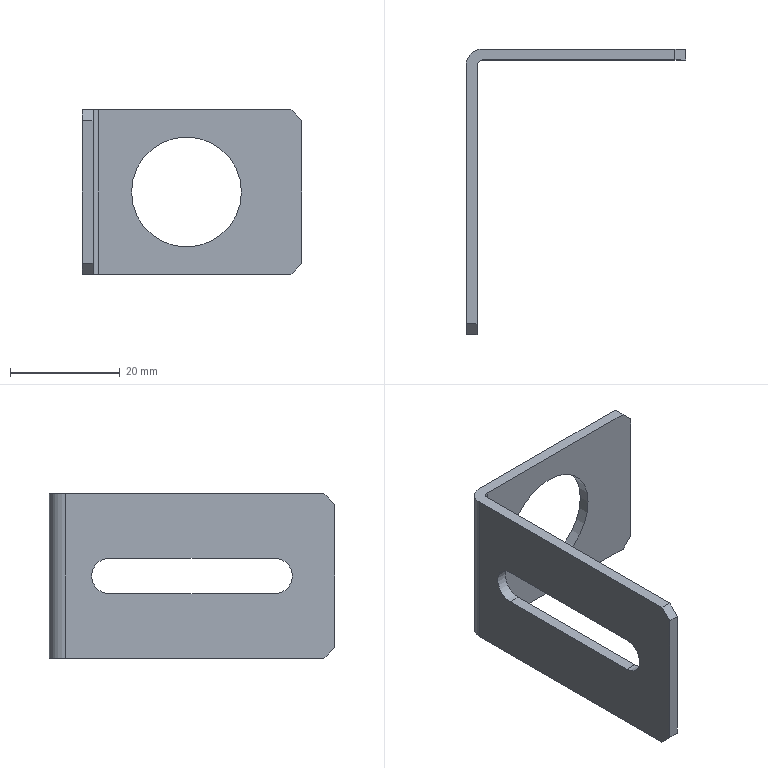Part | SolidWorks | features BaseBody 1 | 1 solid | 20 faces | box 40 x 52 x 30 mm | volume 4248 mm3 | plane 14 | cylinder 6 | commonest cylinder face diameters 6.5 x2 20 x2 2 x1 6 x1
STEP:
#1=CARTESIAN_POINT('',(137.047,1617.079,-1169.));
#2=VERTEX_POINT('',#1);
#3=CARTESIAN_POINT('',(137.047,1617.079,-1149.));
#4=VERTEX_POINT('',#3);
#5=CARTESIAN_POINT('',(137.047,1617.079,-1159.));
#6=DIRECTION('',(0.,1.,0.));
#7=DIRECTION('',(0.,0.,-1.));
#8=AXIS2_PLACEMENT_3D('',#5,#6,#7);
#9=CIRCLE('',#8,10.);
#10=EDGE_CURVE('',#2,#4,#9,.T.);
#11=ORIENTED_EDGE('',*,*,#10,.T.);
#12=CARTESIAN_POINT('',(137.047,1615.079,-1149.));
#13=VERTEX_POINT('',#12);
#14=CARTESIAN_POINT('',(137.047,1665.079,-1149.));
#15=DIRECTION('',(0.,-1.,0.));
#16=VECTOR('',#15,1000.);
#17=LINE('',#14,#16);
#18=EDGE_CURVE('',#4,#13,#17,.T.);
#19=ORIENTED_EDGE('',*,*,#18,.T.);
#20=CARTESIAN_POINT('',(137.047,1615.079,-1169.));
#21=VERTEX_POINT('',#20);
#22=CARTESIAN_POINT('',(137.047,1615.079,-1159.));
#23=DIRECTION('',(0.,-1.,0.));
#24=DIRECTION('',(0.,0.,-1.));
#25=AXIS2_PLACEMENT_3D('',#22,#23,#24);
#26=CIRCLE('',#25,10.);
#27=EDGE_CURVE('',#13,#21,#26,.T.);
#28=ORIENTED_EDGE('',*,*,#27,.T.);
#29=CARTESIAN_POINT('',(137.047,1665.079,-1169.));
#30=DIRECTION('',(0.,-1.,0.));
#31=VECTOR('',#30,1000.);
#32=LINE('',#29,#31);
#33=EDGE_CURVE('',#2,#21,#32,.T.);
#34=ORIENTED_EDGE('',*,*,#33,.F.);
#35=EDGE_LOOP('',(#11,#19,#28,#34));
#36=FACE_OUTER_BOUND('',#35,.T.);
#37=CARTESIAN_POINT('',(137.047,1665.079,-1159.));
#38=DIRECTION('',(0.,-1.,0.));
#39=DIRECTION('',(0.,0.,-1.));
#40=AXIS2_PLACEMENT_3D('',#37,#38,#39);
#41=CYLINDRICAL_SURFACE('',#40,10.);
#42=ADVANCED_FACE('',(#36),#41,.F.);
#43=CARTESIAN_POINT('',(120.047,1606.079,-1155.75));
#44=VERTEX_POINT('',#43);
#45=CARTESIAN_POINT('',(120.047,1576.079,-1155.75));
#46=VERTEX_POINT('',#45);
#47=CARTESIAN_POINT('',(120.047,1565.079,-1155.75));
#48=DIRECTION('',(0.,-1.,0.));
#49=VECTOR('',#48,1000.);
#50=LINE('',#47,#49);
#51=EDGE_CURVE('',#44,#46,#50,.T.);
#52=ORIENTED_EDGE('',*,*,#51,.F.);
#53=CARTESIAN_POINT('',(120.047,1606.079,-1162.25));
#54=VERTEX_POINT('',#53);
#55=CARTESIAN_POINT('',(120.047,1606.079,-1159.));
#56=DIRECTION('',(1.,0.,0.));
#57=DIRECTION('',(0.,0.,-1.));
#58=AXIS2_PLACEMENT_3D('',#55,#56,#57);
#59=CIRCLE('',#58,3.25);
#60=EDGE_CURVE('',#54,#44,#59,.T.);
#61=ORIENTED_EDGE('',*,*,#60,.F.);
#62=CARTESIAN_POINT('',(120.047,1576.079,-1162.25));
#63=VERTEX_POINT('',#62);
#64=CARTESIAN_POINT('',(120.047,1565.079,-1162.25));
#65=DIRECTION('',(0.,1.,0.));
#66=VECTOR('',#65,1000.);
#67=LINE('',#64,#66);
#68=EDGE_CURVE('',#63,#54,#67,.T.);
#69=ORIENTED_EDGE('',*,*,#68,.F.);
#70=CARTESIAN_POINT('',(120.047,1576.079,-1159.));
#71=DIRECTION('',(1.,0.,0.));
#72=DIRECTION('',(0.,0.,-1.));
#73=AXIS2_PLACEMENT_3D('',#70,#71,#72);
#74=CIRCLE('',#73,3.25);
#75=EDGE_CURVE('',#46,#63,#74,.T.);
#76=ORIENTED_EDGE('',*,*,#75,.F.);
#77=EDGE_LOOP('',(#52,#61,#69,#76));
#78=FACE_BOUND('',#77,.T.);
#79=CARTESIAN_POINT('',(120.047,1567.079,-1144.));
#80=VERTEX_POINT('',#79);
#81=CARTESIAN_POINT('',(120.047,1614.079,-1144.));
#82=VERTEX_POINT('',#81);
#83=CARTESIAN_POINT('',(120.047,1565.079,-1144.));
#84=DIRECTION('',(0.,1.,0.));
#85=VECTOR('',#84,1000.);
#86=LINE('',#83,#85);
#87=EDGE_CURVE('',#80,#82,#86,.T.);
#88=ORIENTED_EDGE('',*,*,#87,.F.);
#89=CARTESIAN_POINT('',(120.047,1565.079,-1146.));
#90=VERTEX_POINT('',#89);
#91=CARTESIAN_POINT('',(120.047,1565.079,-1146.));
#92=DIRECTION('',(0.,0.7071,0.7071));
#93=VECTOR('',#92,1000.);
#94=LINE('',#91,#93);
#95=EDGE_CURVE('',#90,#80,#94,.T.);
#96=ORIENTED_EDGE('',*,*,#95,.F.);
#97=CARTESIAN_POINT('',(120.047,1565.079,-1172.));
#98=VERTEX_POINT('',#97);
#99=CARTESIAN_POINT('',(120.047,1565.079,-1174.));
#100=DIRECTION('',(0.,0.,1.));
#101=VECTOR('',#100,1000.);
#102=LINE('',#99,#101);
#103=EDGE_CURVE('',#98,#90,#102,.T.);
#104=ORIENTED_EDGE('',*,*,#103,.F.);
#105=CARTESIAN_POINT('',(120.047,1567.079,-1174.));
#106=VERTEX_POINT('',#105);
#107=CARTESIAN_POINT('',(120.047,1567.079,-1174.));
#108=DIRECTION('',(0.,-0.7071,0.7071));
#109=VECTOR('',#108,1000.);
#110=LINE('',#107,#109);
#111=EDGE_CURVE('',#106,#98,#110,.T.);
#112=ORIENTED_EDGE('',*,*,#111,.F.);
#113=CARTESIAN_POINT('',(120.047,1614.079,-1174.));
#114=VERTEX_POINT('',#113);
#115=CARTESIAN_POINT('',(120.047,1565.079,-1174.));
#116=DIRECTION('',(0.,-1.,0.));
#117=VECTOR('',#116,1000.);
#118=LINE('',#115,#117);
#119=EDGE_CURVE('',#114,#106,#118,.T.);
#120=ORIENTED_EDGE('',*,*,#119,.F.);
#121=CARTESIAN_POINT('',(120.047,1614.079,-1174.));
#122=DIRECTION('',(0.,0.,-1.));
#123=VECTOR('',#122,1000.);
#124=LINE('',#121,#123);
#125=EDGE_CURVE('',#82,#114,#124,.T.);
#126=ORIENTED_EDGE('',*,*,#125,.F.);
#127=EDGE_LOOP('',(#88,#96,#104,#112,#120,#126));
#128=FACE_OUTER_BOUND('',#127,.T.);
#129=CARTESIAN_POINT('',(120.047,1565.079,-1174.));
#130=DIRECTION('',(-1.,0.,0.));
#131=DIRECTION('',(0.,0.,1.));
#132=AXIS2_PLACEMENT_3D('',#129,#130,#131);
#133=PLANE('',#132);
#134=ADVANCED_FACE('',(#78,#128),#133,.F.);
#135=CARTESIAN_POINT('',(118.047,1576.079,-1162.25));
#136=VERTEX_POINT('',#135);
#137=CARTESIAN_POINT('',(110.047,1576.079,-1162.25));
#138=DIRECTION('',(1.,0.,0.));
#139=VECTOR('',#138,1000.);
#140=LINE('',#137,#139);
#141=EDGE_CURVE('',#136,#63,#140,.T.);
#142=ORIENTED_EDGE('',*,*,#141,.F.);
#143=CARTESIAN_POINT('',(118.047,1576.079,-1155.75));
#144=VERTEX_POINT('',#143);
#145=CARTESIAN_POINT('',(118.047,1576.079,-1159.));
#146=DIRECTION('',(1.,0.,0.));
#147=DIRECTION('',(0.,0.,-1.));
#148=AXIS2_PLACEMENT_3D('',#145,#146,#147);
#149=CIRCLE('',#148,3.25);
#150=EDGE_CURVE('',#144,#136,#149,.T.);
#151=ORIENTED_EDGE('',*,*,#150,.F.);
#152=CARTESIAN_POINT('',(110.047,1576.079,-1155.75));
#153=DIRECTION('',(-1.,0.,0.));
#154=VECTOR('',#153,1000.);
#155=LINE('',#152,#154);
#156=EDGE_CURVE('',#46,#144,#155,.T.);
#157=ORIENTED_EDGE('',*,*,#156,.F.);
#158=ORIENTED_EDGE('',*,*,#75,.T.);
#159=EDGE_LOOP('',(#142,#151,#157,#158));
#160=FACE_OUTER_BOUND('',#159,.T.);
#161=CARTESIAN_POINT('',(110.047,1576.079,-1159.));
#162=DIRECTION('',(1.,0.,0.));
#163=DIRECTION('',(0.,0.,-1.));
#164=AXIS2_PLACEMENT_3D('',#161,#162,#163);
#165=CYLINDRICAL_SURFACE('',#164,3.25);
#166=ADVANCED_FACE('',(#160),#165,.F.);
#167=ORIENTED_EDGE('',*,*,#156,.T.);
#168=CARTESIAN_POINT('',(118.047,1606.079,-1155.75));
#169=VERTEX_POINT('',#168);
#170=CARTESIAN_POINT('',(118.047,1576.079,-1155.75));
#171=DIRECTION('',(0.,-1.,0.));
#172=VECTOR('',#171,1000.);
#173=LINE('',#170,#172);
#174=EDGE_CURVE('',#169,#144,#173,.T.);
#175=ORIENTED_EDGE('',*,*,#174,.F.);
#176=CARTESIAN_POINT('',(110.047,1606.079,-1155.75));
#177=DIRECTION('',(-1.,0.,0.));
#178=VECTOR('',#177,1000.);
#179=LINE('',#176,#178);
#180=EDGE_CURVE('',#44,#169,#179,.T.);
#181=ORIENTED_EDGE('',*,*,#180,.F.);
#182=ORIENTED_EDGE('',*,*,#51,.T.);
#183=EDGE_LOOP('',(#167,#175,#181,#182));
#184=FACE_OUTER_BOUND('',#183,.T.);
#185=CARTESIAN_POINT('',(110.047,1576.079,-1155.75));
#186=DIRECTION('',(0.,0.,1.));
#187=DIRECTION('',(1.,0.,0.));
#188=AXIS2_PLACEMENT_3D('',#185,#186,#187);
#189=PLANE('',#188);
#190=ADVANCED_FACE('',(#184),#189,.F.);
#191=ORIENTED_EDGE('',*,*,#180,.T.);
#192=CARTESIAN_POINT('',(118.047,1606.079,-1162.25));
#193=VERTEX_POINT('',#192);
#194=CARTESIAN_POINT('',(118.047,1606.079,-1159.));
#195=DIRECTION('',(1.,0.,0.));
#196=DIRECTION('',(0.,0.,-1.));
#197=AXIS2_PLACEMENT_3D('',#194,#195,#196);
#198=CIRCLE('',#197,3.25);
#199=EDGE_CURVE('',#193,#169,#198,.T.);
#200=ORIENTED_EDGE('',*,*,#199,.F.);
#201=CARTESIAN_POINT('',(110.047,1606.079,-1162.25));
#202=DIRECTION('',(-1.,0.,0.));
#203=VECTOR('',#202,1000.);
#204=LINE('',#201,#203);
#205=EDGE_CURVE('',#54,#193,#204,.T.);
#206=ORIENTED_EDGE('',*,*,#205,.F.);
#207=ORIENTED_EDGE('',*,*,#60,.T.);
#208=EDGE_LOOP('',(#191,#200,#206,#207));
#209=FACE_OUTER_BOUND('',#208,.T.);
#210=CARTESIAN_POINT('',(110.047,1606.079,-1159.));
#211=DIRECTION('',(1.,0.,0.));
#212=DIRECTION('',(0.,0.,-1.));
#213=AXIS2_PLACEMENT_3D('',#210,#211,#212);
#214=CYLINDRICAL_SURFACE('',#213,3.25);
#215=ADVANCED_FACE('',(#209),#214,.F.);
#216=ORIENTED_EDGE('',*,*,#205,.T.);
#217=CARTESIAN_POINT('',(118.047,1576.079,-1162.25));
#218=DIRECTION('',(0.,1.,0.));
#219=VECTOR('',#218,1000.);
#220=LINE('',#217,#219);
#221=EDGE_CURVE('',#136,#193,#220,.T.);
#222=ORIENTED_EDGE('',*,*,#221,.F.);
#223=ORIENTED_EDGE('',*,*,#141,.T.);
#224=ORIENTED_EDGE('',*,*,#68,.T.);
#225=EDGE_LOOP('',(#216,#222,#223,#224));
#226=FACE_OUTER_BOUND('',#225,.T.);
#227=CARTESIAN_POINT('',(110.047,1576.079,-1162.25));
#228=DIRECTION('',(0.,0.,-1.));
#229=DIRECTION('',(-1.,0.,0.));
#230=AXIS2_PLACEMENT_3D('',#227,#228,#229);
#231=PLANE('',#230);
#232=ADVANCED_FACE('',(#226),#231,.F.);
#233=CARTESIAN_POINT('',(121.047,1615.079,-1144.));
#234=VERTEX_POINT('',#233);
#235=CARTESIAN_POINT('',(121.047,1614.079,-1144.));
#236=DIRECTION('',(0.,0.,-1.));
#237=DIRECTION('',(-1.,0.,0.));
#238=AXIS2_PLACEMENT_3D('',#235,#236,#237);
#239=CIRCLE('',#238,1.);
#240=EDGE_CURVE('',#82,#234,#239,.T.);
#241=ORIENTED_EDGE('',*,*,#240,.F.);
#242=ORIENTED_EDGE('',*,*,#125,.T.);
#243=CARTESIAN_POINT('',(121.047,1615.079,-1174.));
#244=VERTEX_POINT('',#243);
#245=CARTESIAN_POINT('',(121.047,1614.079,-1174.));
#246=DIRECTION('',(0.,0.,1.));
#247=DIRECTION('',(-1.,0.,0.));
#248=AXIS2_PLACEMENT_3D('',#245,#246,#247);
#249=CIRCLE('',#248,1.);
#250=EDGE_CURVE('',#244,#114,#249,.T.);
#251=ORIENTED_EDGE('',*,*,#250,.F.);
#252=CARTESIAN_POINT('',(121.047,1615.079,-1174.));
#253=DIRECTION('',(0.,0.,-1.));
#254=VECTOR('',#253,1000.);
#255=LINE('',#252,#254);
#256=EDGE_CURVE('',#234,#244,#255,.T.);
#257=ORIENTED_EDGE('',*,*,#256,.F.);
#258=EDGE_LOOP('',(#241,#242,#251,#257));
#259=FACE_OUTER_BOUND('',#258,.T.);
#260=CARTESIAN_POINT('',(121.047,1614.079,-1174.));
#261=DIRECTION('',(0.,0.,-1.));
#262=DIRECTION('',(-1.,0.,0.));
#263=AXIS2_PLACEMENT_3D('',#260,#261,#262);
#264=CYLINDRICAL_SURFACE('',#263,1.);
#265=ADVANCED_FACE('',(#259),#264,.F.);
#266=CARTESIAN_POINT('',(118.047,1567.079,-1144.));
#267=VERTEX_POINT('',#266);
#268=CARTESIAN_POINT('',(118.047,1614.079,-1144.));
#269=VERTEX_POINT('',#268);
#270=CARTESIAN_POINT('',(118.047,1615.079,-1144.));
#271=DIRECTION('',(0.,1.,0.));
#272=VECTOR('',#271,1000.);
#273=LINE('',#270,#272);
#274=EDGE_CURVE('',#267,#269,#273,.T.);
#275=ORIENTED_EDGE('',*,*,#274,.F.);
#276=CARTESIAN_POINT('',(158.047,1567.079,-1144.));
#277=DIRECTION('',(-1.,0.,0.));
#278=VECTOR('',#277,1000.);
#279=LINE('',#276,#278);
#280=EDGE_CURVE('',#80,#267,#279,.T.);
#281=ORIENTED_EDGE('',*,*,#280,.F.);
#282=ORIENTED_EDGE('',*,*,#87,.T.);
#283=ORIENTED_EDGE('',*,*,#240,.T.);
#284=CARTESIAN_POINT('',(156.047,1615.079,-1144.));
#285=VERTEX_POINT('',#284);
#286=CARTESIAN_POINT('',(158.047,1615.079,-1144.));
#287=DIRECTION('',(-1.,0.,0.));
#288=VECTOR('',#287,1000.);
#289=LINE('',#286,#288);
#290=EDGE_CURVE('',#285,#234,#289,.T.);
#291=ORIENTED_EDGE('',*,*,#290,.F.);
#292=CARTESIAN_POINT('',(156.047,1617.079,-1144.));
#293=VERTEX_POINT('',#292);
#294=CARTESIAN_POINT('',(156.047,1615.079,-1144.));
#295=DIRECTION('',(0.,-1.,0.));
#296=VECTOR('',#295,1000.);
#297=LINE('',#294,#296);
#298=EDGE_CURVE('',#293,#285,#297,.T.);
#299=ORIENTED_EDGE('',*,*,#298,.F.);
#300=CARTESIAN_POINT('',(121.047,1617.079,-1144.));
#301=VERTEX_POINT('',#300);
#302=CARTESIAN_POINT('',(158.047,1617.079,-1144.));
#303=DIRECTION('',(1.,0.,0.));
#304=VECTOR('',#303,1000.);
#305=LINE('',#302,#304);
#306=EDGE_CURVE('',#301,#293,#305,.T.);
#307=ORIENTED_EDGE('',*,*,#306,.F.);
#308=CARTESIAN_POINT('',(121.047,1614.079,-1144.));
#309=DIRECTION('',(0.,0.,-1.));
#310=DIRECTION('',(1.,0.,0.));
#311=AXIS2_PLACEMENT_3D('',#308,#309,#310);
#312=CIRCLE('',#311,3.);
#313=EDGE_CURVE('',#269,#301,#312,.T.);
#314=ORIENTED_EDGE('',*,*,#313,.F.);
#315=EDGE_LOOP('',(#275,#281,#282,#283,#291,#299,#307,#314));
#316=FACE_OUTER_BOUND('',#315,.T.);
#317=CARTESIAN_POINT('',(158.047,1615.079,-1144.));
#318=DIRECTION('',(0.,0.,-1.));
#319=DIRECTION('',(-1.,0.,0.));
#320=AXIS2_PLACEMENT_3D('',#317,#318,#319);
#321=PLANE('',#320);
#322=ADVANCED_FACE('',(#316),#321,.F.);
#323=CARTESIAN_POINT('',(118.047,1565.079,-1146.));
#324=VERTEX_POINT('',#323);
#325=CARTESIAN_POINT('',(120.047,1565.079,-1146.));
#326=DIRECTION('',(1.,0.,0.));
#327=VECTOR('',#326,1000.);
#328=LINE('',#325,#327);
#329=EDGE_CURVE('',#324,#90,#328,.T.);
#330=ORIENTED_EDGE('',*,*,#329,.T.);
#331=ORIENTED_EDGE('',*,*,#95,.T.);
#332=ORIENTED_EDGE('',*,*,#280,.T.);
#333=CARTESIAN_POINT('',(118.047,1565.079,-1146.));
#334=DIRECTION('',(0.,-0.7071,-0.7071));
#335=VECTOR('',#334,1000.);
#336=LINE('',#333,#335);
#337=EDGE_CURVE('',#267,#324,#336,.T.);
#338=ORIENTED_EDGE('',*,*,#337,.T.);
#339=EDGE_LOOP('',(#330,#331,#332,#338));
#340=FACE_OUTER_BOUND('',#339,.T.);
#341=CARTESIAN_POINT('',(120.047,1565.079,-1146.));
#342=DIRECTION('',(0.,-0.7071,0.7071));
#343=DIRECTION('',(0.,-0.7071,-0.7071));
#344=AXIS2_PLACEMENT_3D('',#341,#342,#343);
#345=PLANE('',#344);
#346=ADVANCED_FACE('',(#340),#345,.T.);
#347=CARTESIAN_POINT('',(118.047,1565.079,-1172.));
#348=VERTEX_POINT('',#347);
#349=CARTESIAN_POINT('',(120.047,1565.079,-1172.));
#350=DIRECTION('',(1.,0.,0.));
#351=VECTOR('',#350,1000.);
#352=LINE('',#349,#351);
#353=EDGE_CURVE('',#348,#98,#352,.T.);
#354=ORIENTED_EDGE('',*,*,#353,.T.);
#355=ORIENTED_EDGE('',*,*,#103,.T.);
#356=ORIENTED_EDGE('',*,*,#329,.F.);
#357=CARTESIAN_POINT('',(118.047,1565.079,-1174.));
#358=DIRECTION('',(0.,0.,-1.));
#359=VECTOR('',#358,1000.);
#360=LINE('',#357,#359);
#361=EDGE_CURVE('',#324,#348,#360,.T.);
#362=ORIENTED_EDGE('',*,*,#361,.T.);
#363=EDGE_LOOP('',(#354,#355,#356,#362));
#364=FACE_OUTER_BOUND('',#363,.T.);
#365=CARTESIAN_POINT('',(120.047,1565.079,-1174.));
#366=DIRECTION('',(0.,-1.,0.));
#367=DIRECTION('',(0.,0.,-1.));
#368=AXIS2_PLACEMENT_3D('',#365,#366,#367);
#369=PLANE('',#368);
#370=ADVANCED_FACE('',(#364),#369,.T.);
#371=ORIENTED_EDGE('',*,*,#353,.F.);
#372=CARTESIAN_POINT('',(118.047,1567.079,-1174.));
#373=VERTEX_POINT('',#372);
#374=CARTESIAN_POINT('',(118.047,1565.079,-1172.));
#375=DIRECTION('',(0.,0.7071,-0.7071));
#376=VECTOR('',#375,1000.);
#377=LINE('',#374,#376);
#378=EDGE_CURVE('',#348,#373,#377,.T.);
#379=ORIENTED_EDGE('',*,*,#378,.T.);
#380=CARTESIAN_POINT('',(120.047,1567.079,-1174.));
#381=DIRECTION('',(1.,0.,0.));
#382=VECTOR('',#381,1000.);
#383=LINE('',#380,#382);
#384=EDGE_CURVE('',#373,#106,#383,.T.);
#385=ORIENTED_EDGE('',*,*,#384,.T.);
#386=ORIENTED_EDGE('',*,*,#111,.T.);
#387=EDGE_LOOP('',(#371,#379,#385,#386));
#388=FACE_OUTER_BOUND('',#387,.T.);
#389=CARTESIAN_POINT('',(120.047,1565.079,-1172.));
#390=DIRECTION('',(0.,-0.7071,-0.7071));
#391=DIRECTION('',(0.,0.7071,-0.7071));
#392=AXIS2_PLACEMENT_3D('',#389,#390,#391);
#393=PLANE('',#392);
#394=ADVANCED_FACE('',(#388),#393,.T.);
#395=CARTESIAN_POINT('',(156.047,1617.079,-1174.));
#396=VERTEX_POINT('',#395);
#397=CARTESIAN_POINT('',(121.047,1617.079,-1174.));
#398=VERTEX_POINT('',#397);
#399=CARTESIAN_POINT('',(158.047,1617.079,-1174.));
#400=DIRECTION('',(-1.,0.,0.));
#401=VECTOR('',#400,1000.);
#402=LINE('',#399,#401);
#403=EDGE_CURVE('',#396,#398,#402,.T.);
#404=ORIENTED_EDGE('',*,*,#403,.F.);
#405=CARTESIAN_POINT('',(156.047,1615.079,-1174.));
#406=VERTEX_POINT('',#405);
#407=CARTESIAN_POINT('',(156.047,1615.079,-1174.));
#408=DIRECTION('',(0.,1.,0.));
#409=VECTOR('',#408,1000.);
#410=LINE('',#407,#409);
#411=EDGE_CURVE('',#406,#396,#410,.T.);
#412=ORIENTED_EDGE('',*,*,#411,.F.);
#413=CARTESIAN_POINT('',(158.047,1615.079,-1174.));
#414=DIRECTION('',(1.,0.,0.));
#415=VECTOR('',#414,1000.);
#416=LINE('',#413,#415);
#417=EDGE_CURVE('',#244,#406,#416,.T.);
#418=ORIENTED_EDGE('',*,*,#417,.F.);
#419=ORIENTED_EDGE('',*,*,#250,.T.);
#420=ORIENTED_EDGE('',*,*,#119,.T.);
#421=ORIENTED_EDGE('',*,*,#384,.F.);
#422=CARTESIAN_POINT('',(118.047,1614.079,-1174.));
#423=VERTEX_POINT('',#422);
#424=CARTESIAN_POINT('',(118.047,1615.079,-1174.));
#425=DIRECTION('',(0.,-1.,0.));
#426=VECTOR('',#425,1000.);
#427=LINE('',#424,#426);
#428=EDGE_CURVE('',#423,#373,#427,.T.);
#429=ORIENTED_EDGE('',*,*,#428,.F.);
#430=CARTESIAN_POINT('',(121.047,1614.079,-1174.));
#431=DIRECTION('',(0.,0.,1.));
#432=DIRECTION('',(1.,0.,0.));
#433=AXIS2_PLACEMENT_3D('',#430,#431,#432);
#434=CIRCLE('',#433,3.);
#435=EDGE_CURVE('',#398,#423,#434,.T.);
#436=ORIENTED_EDGE('',*,*,#435,.F.);
#437=EDGE_LOOP('',(#404,#412,#418,#419,#420,#421,#429,#436));
#438=FACE_OUTER_BOUND('',#437,.T.);
#439=CARTESIAN_POINT('',(158.047,1615.079,-1174.));
#440=DIRECTION('',(0.,0.,1.));
#441=DIRECTION('',(1.,0.,0.));
#442=AXIS2_PLACEMENT_3D('',#439,#440,#441);
#443=PLANE('',#442);
#444=ADVANCED_FACE('',(#438),#443,.F.);
#445=ORIENTED_EDGE('',*,*,#221,.T.);
#446=ORIENTED_EDGE('',*,*,#199,.T.);
#447=ORIENTED_EDGE('',*,*,#174,.T.);
#448=ORIENTED_EDGE('',*,*,#150,.T.);
#449=EDGE_LOOP('',(#445,#446,#447,#448));
#450=FACE_BOUND('',#449,.T.);
#451=ORIENTED_EDGE('',*,*,#428,.T.);
#452=ORIENTED_EDGE('',*,*,#378,.F.);
#453=ORIENTED_EDGE('',*,*,#361,.F.);
#454=ORIENTED_EDGE('',*,*,#337,.F.);
#455=ORIENTED_EDGE('',*,*,#274,.T.);
#456=CARTESIAN_POINT('',(118.047,1614.079,-1174.));
#457=DIRECTION('',(0.,0.,1.));
#458=VECTOR('',#457,1000.);
#459=LINE('',#456,#458);
#460=EDGE_CURVE('',#423,#269,#459,.T.);
#461=ORIENTED_EDGE('',*,*,#460,.F.);
#462=EDGE_LOOP('',(#451,#452,#453,#454,#455,#461));
#463=FACE_OUTER_BOUND('',#462,.T.);
#464=CARTESIAN_POINT('',(118.047,1617.079,-1174.));
#465=DIRECTION('',(1.,0.,0.));
#466=DIRECTION('',(0.,0.,-1.));
#467=AXIS2_PLACEMENT_3D('',#464,#465,#466);
#468=PLANE('',#467);
#469=ADVANCED_FACE('',(#450,#463),#468,.F.);
#470=CARTESIAN_POINT('',(137.047,1615.079,-1159.));
#471=DIRECTION('',(0.,-1.,0.));
#472=DIRECTION('',(0.,0.,-1.));
#473=AXIS2_PLACEMENT_3D('',#470,#471,#472);
#474=CIRCLE('',#473,10.);
#475=EDGE_CURVE('',#21,#13,#474,.T.);
#476=ORIENTED_EDGE('',*,*,#475,.F.);
#477=ORIENTED_EDGE('',*,*,#27,.F.);
#478=EDGE_LOOP('',(#476,#477));
#479=FACE_BOUND('',#478,.T.);
#480=ORIENTED_EDGE('',*,*,#417,.T.);
#481=CARTESIAN_POINT('',(158.047,1615.079,-1172.));
#482=VERTEX_POINT('',#481);
#483=CARTESIAN_POINT('',(158.047,1615.079,-1172.));
#484=DIRECTION('',(-0.7071,0.,-0.7071));
#485=VECTOR('',#484,1000.);
#486=LINE('',#483,#485);
#487=EDGE_CURVE('',#482,#406,#486,.T.);
#488=ORIENTED_EDGE('',*,*,#487,.F.);
#489=CARTESIAN_POINT('',(158.047,1615.079,-1146.));
#490=VERTEX_POINT('',#489);
#491=CARTESIAN_POINT('',(158.047,1615.079,-1174.));
#492=DIRECTION('',(0.,0.,-1.));
#493=VECTOR('',#492,1000.);
#494=LINE('',#491,#493);
#495=EDGE_CURVE('',#490,#482,#494,.T.);
#496=ORIENTED_EDGE('',*,*,#495,.F.);
#497=CARTESIAN_POINT('',(156.047,1615.079,-1144.));
#498=DIRECTION('',(0.7071,0.,-0.7071));
#499=VECTOR('',#498,1000.);
#500=LINE('',#497,#499);
#501=EDGE_CURVE('',#285,#490,#500,.T.);
#502=ORIENTED_EDGE('',*,*,#501,.F.);
#503=ORIENTED_EDGE('',*,*,#290,.T.);
#504=ORIENTED_EDGE('',*,*,#256,.T.);
#505=EDGE_LOOP('',(#480,#488,#496,#502,#503,#504));
#506=FACE_OUTER_BOUND('',#505,.T.);
#507=CARTESIAN_POINT('',(158.047,1615.079,-1174.));
#508=DIRECTION('',(0.,1.,0.));
#509=DIRECTION('',(0.,0.,1.));
#510=AXIS2_PLACEMENT_3D('',#507,#508,#509);
#511=PLANE('',#510);
#512=ADVANCED_FACE('',(#479,#506),#511,.F.);
#513=CARTESIAN_POINT('',(121.047,1617.079,-1174.));
#514=DIRECTION('',(0.,0.,-1.));
#515=VECTOR('',#514,1000.);
#516=LINE('',#513,#515);
#517=EDGE_CURVE('',#301,#398,#516,.T.);
#518=ORIENTED_EDGE('',*,*,#517,.T.);
#519=ORIENTED_EDGE('',*,*,#435,.T.);
#520=ORIENTED_EDGE('',*,*,#460,.T.);
#521=ORIENTED_EDGE('',*,*,#313,.T.);
#522=EDGE_LOOP('',(#518,#519,#520,#521));
#523=FACE_OUTER_BOUND('',#522,.T.);
#524=CARTESIAN_POINT('',(121.047,1614.079,-1174.));
#525=DIRECTION('',(0.,0.,1.));
#526=DIRECTION('',(1.,0.,0.));
#527=AXIS2_PLACEMENT_3D('',#524,#525,#526);
#528=CYLINDRICAL_SURFACE('',#527,3.);
#529=ADVANCED_FACE('',(#523),#528,.T.);
#530=CARTESIAN_POINT('',(158.047,1617.079,-1146.));
#531=VERTEX_POINT('',#530);
#532=CARTESIAN_POINT('',(158.047,1617.079,-1146.));
#533=DIRECTION('',(0.,1.,0.));
#534=VECTOR('',#533,1000.);
#535=LINE('',#532,#534);
#536=EDGE_CURVE('',#490,#531,#535,.T.);
#537=ORIENTED_EDGE('',*,*,#536,.T.);
#538=CARTESIAN_POINT('',(158.047,1617.079,-1146.));
#539=DIRECTION('',(-0.7071,0.,0.7071));
#540=VECTOR('',#539,1000.);
#541=LINE('',#538,#540);
#542=EDGE_CURVE('',#531,#293,#541,.T.);
#543=ORIENTED_EDGE('',*,*,#542,.T.);
#544=ORIENTED_EDGE('',*,*,#298,.T.);
#545=ORIENTED_EDGE('',*,*,#501,.T.);
#546=EDGE_LOOP('',(#537,#543,#544,#545));
#547=FACE_OUTER_BOUND('',#546,.T.);
#548=CARTESIAN_POINT('',(158.047,1617.079,-1146.));
#549=DIRECTION('',(0.7071,0.,0.7071));
#550=DIRECTION('',(0.7071,0.,-0.7071));
#551=AXIS2_PLACEMENT_3D('',#548,#549,#550);
#552=PLANE('',#551);
#553=ADVANCED_FACE('',(#547),#552,.T.);
#554=ORIENTED_EDGE('',*,*,#10,.F.);
#555=CARTESIAN_POINT('',(137.047,1617.079,-1159.));
#556=DIRECTION('',(0.,1.,0.));
#557=DIRECTION('',(0.,0.,-1.));
#558=AXIS2_PLACEMENT_3D('',#555,#556,#557);
#559=CIRCLE('',#558,10.);
#560=EDGE_CURVE('',#4,#2,#559,.T.);
#561=ORIENTED_EDGE('',*,*,#560,.F.);
#562=EDGE_LOOP('',(#554,#561));
#563=FACE_BOUND('',#562,.T.);
#564=ORIENTED_EDGE('',*,*,#306,.T.);
#565=ORIENTED_EDGE('',*,*,#542,.F.);
#566=CARTESIAN_POINT('',(158.047,1617.079,-1172.));
#567=VERTEX_POINT('',#566);
#568=CARTESIAN_POINT('',(158.047,1617.079,-1174.));
#569=DIRECTION('',(0.,0.,1.));
#570=VECTOR('',#569,1000.);
#571=LINE('',#568,#570);
#572=EDGE_CURVE('',#567,#531,#571,.T.);
#573=ORIENTED_EDGE('',*,*,#572,.F.);
#574=CARTESIAN_POINT('',(156.047,1617.079,-1174.));
#575=DIRECTION('',(0.7071,0.,0.7071));
#576=VECTOR('',#575,1000.);
#577=LINE('',#574,#576);
#578=EDGE_CURVE('',#396,#567,#577,.T.);
#579=ORIENTED_EDGE('',*,*,#578,.F.);
#580=ORIENTED_EDGE('',*,*,#403,.T.);
#581=ORIENTED_EDGE('',*,*,#517,.F.);
#582=EDGE_LOOP('',(#564,#565,#573,#579,#580,#581));
#583=FACE_OUTER_BOUND('',#582,.T.);
#584=CARTESIAN_POINT('',(158.047,1617.079,-1174.));
#585=DIRECTION('',(0.,-1.,0.));
#586=DIRECTION('',(0.,0.,-1.));
#587=AXIS2_PLACEMENT_3D('',#584,#585,#586);
#588=PLANE('',#587);
#589=ADVANCED_FACE('',(#563,#583),#588,.F.);
#590=CARTESIAN_POINT('',(158.047,1617.079,-1172.));
#591=DIRECTION('',(0.,-1.,0.));
#592=VECTOR('',#591,1000.);
#593=LINE('',#590,#592);
#594=EDGE_CURVE('',#567,#482,#593,.T.);
#595=ORIENTED_EDGE('',*,*,#594,.T.);
#596=ORIENTED_EDGE('',*,*,#487,.T.);
#597=ORIENTED_EDGE('',*,*,#411,.T.);
#598=ORIENTED_EDGE('',*,*,#578,.T.);
#599=EDGE_LOOP('',(#595,#596,#597,#598));
#600=FACE_OUTER_BOUND('',#599,.T.);
#601=CARTESIAN_POINT('',(158.047,1617.079,-1172.));
#602=DIRECTION('',(0.7071,0.,-0.7071));
#603=DIRECTION('',(-0.7071,0.,-0.7071));
#604=AXIS2_PLACEMENT_3D('',#601,#602,#603);
#605=PLANE('',#604);
#606=ADVANCED_FACE('',(#600),#605,.T.);
#607=ORIENTED_EDGE('',*,*,#18,.F.);
#608=ORIENTED_EDGE('',*,*,#560,.T.);
#609=ORIENTED_EDGE('',*,*,#33,.T.);
#610=ORIENTED_EDGE('',*,*,#475,.T.);
#611=EDGE_LOOP('',(#607,#608,#609,#610));
#612=FACE_OUTER_BOUND('',#611,.T.);
#613=CARTESIAN_POINT('',(137.047,1665.079,-1159.));
#614=DIRECTION('',(0.,-1.,0.));
#615=DIRECTION('',(0.,0.,-1.));
#616=AXIS2_PLACEMENT_3D('',#613,#614,#615);
#617=CYLINDRICAL_SURFACE('',#616,10.);
#618=ADVANCED_FACE('',(#612),#617,.F.);
#619=ORIENTED_EDGE('',*,*,#536,.F.);
#620=ORIENTED_EDGE('',*,*,#495,.T.);
#621=ORIENTED_EDGE('',*,*,#594,.F.);
#622=ORIENTED_EDGE('',*,*,#572,.T.);
#623=EDGE_LOOP('',(#619,#620,#621,#622));
#624=FACE_OUTER_BOUND('',#623,.T.);
#625=CARTESIAN_POINT('',(158.047,1617.079,-1174.));
#626=DIRECTION('',(1.,0.,0.));
#627=DIRECTION('',(0.,0.,-1.));
#628=AXIS2_PLACEMENT_3D('',#625,#626,#627);
#629=PLANE('',#628);
#630=ADVANCED_FACE('',(#624),#629,.T.);
#631=CLOSED_SHELL('',(#42,#134,#166,#190,#215,#232,#265,#322,#346,#370,#394,#444,#469,#512,#529,#553,#589,#606,#618,#630));
#632=MANIFOLD_SOLID_BREP('',#631);
#633=CARTESIAN_POINT('',(0.,0.,0.));
#634=DIRECTION('',(0.,0.,1.));
#635=DIRECTION('',(1.,0.,0.));
#636=AXIS2_PLACEMENT_3D('',#633,#634,#635);
#637=(LENGTH_UNIT()NAMED_UNIT(*)SI_UNIT(.MILLI.,.METRE.));
#638=UNCERTAINTY_MEASURE_WITH_UNIT(LENGTH_MEASURE(0.00001),#637,'','');
#639=(NAMED_UNIT(*)PLANE_ANGLE_UNIT()SI_UNIT($,.RADIAN.));
#640=(NAMED_UNIT(*)SI_UNIT($,.STERADIAN.)SOLID_ANGLE_UNIT());
#641=(GEOMETRIC_REPRESENTATION_CONTEXT(3)GLOBAL_UNCERTAINTY_ASSIGNED_CONTEXT((#638))GLOBAL_UNIT_ASSIGNED_CONTEXT((#637,#639,#640))REPRESENTATION_CONTEXT('',''));
#642=ADVANCED_BREP_SHAPE_REPRESENTATION('',(#632,#636),#641);